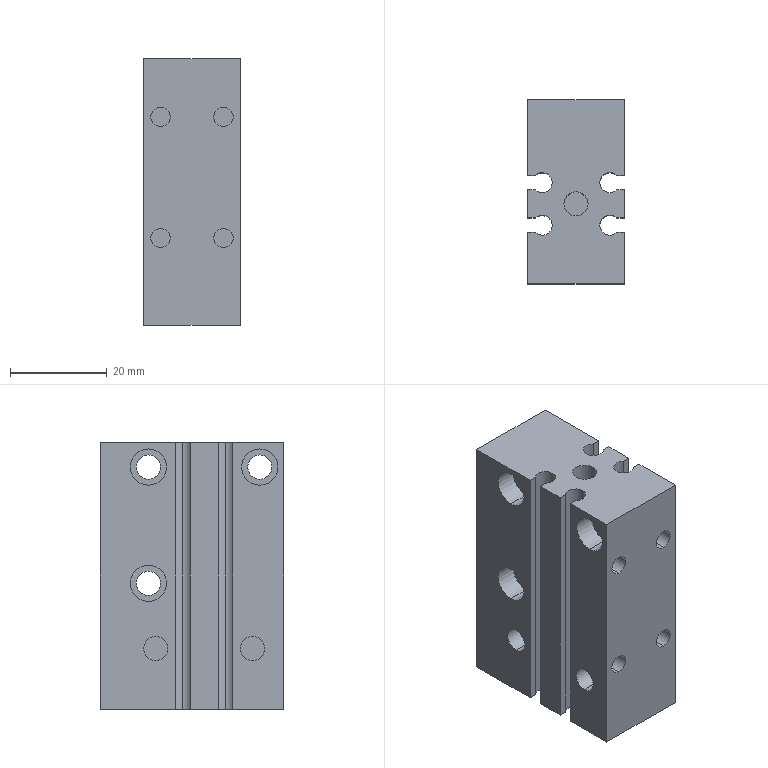Part | NX | 1 solid | 96 faces | box 20 x 38 x 55 mm | volume 32885 mm3 | cylinder 56 | plane 40 | commonest cylinder face diameters 5 x20 4 x16 7.5 x12 4.15 x6 10 x2